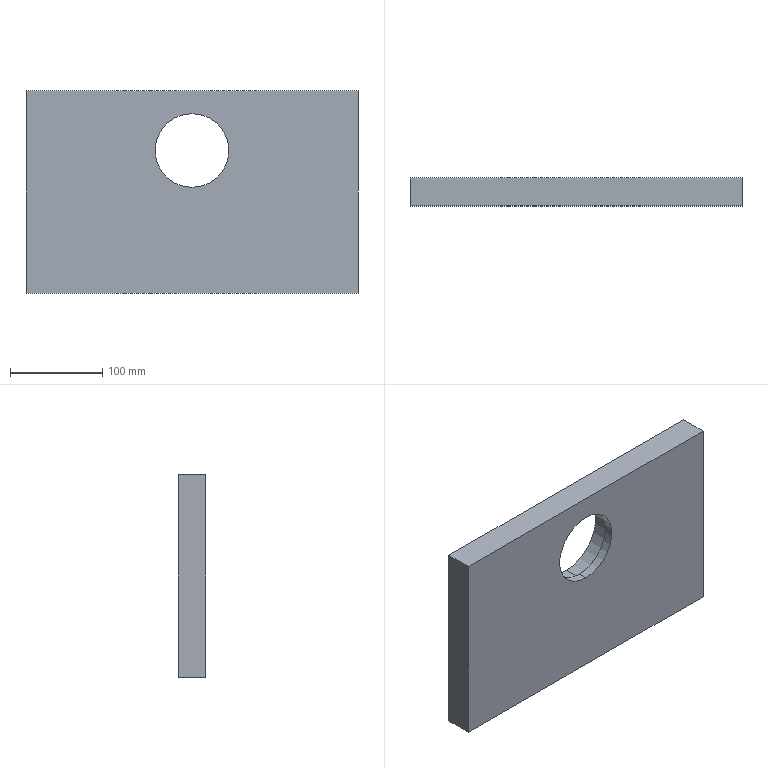Part | SolidWorks | features Cut 2, Extrusion 1 | 1 solid | 11 faces | box 360 x 30 x 220 mm | volume 2198500 mm3 | plane 7 | cylinder 4 | commonest cylinder face diameters 80 x2 90 x2
STEP:
#1=CARTESIAN_POINT('',(0.,10.,90.));
#2=VERTEX_POINT('',#1);
#3=CARTESIAN_POINT('',(0.,10.,0.));
#4=VERTEX_POINT('',#3);
#5=CARTESIAN_POINT('',(0.,10.,45.));
#6=DIRECTION('',(0.,-1.,0.));
#7=DIRECTION('',(0.,0.,-1.));
#8=AXIS2_PLACEMENT_3D('',#5,#6,#7);
#9=CIRCLE('',#8,45.);
#10=EDGE_CURVE('',#2,#4,#9,.T.);
#11=ORIENTED_EDGE('',*,*,#10,.T.);
#12=CARTESIAN_POINT('',(0.,30.,0.));
#13=VERTEX_POINT('',#12);
#14=CARTESIAN_POINT('',(0.,10.,0.));
#15=DIRECTION('',(0.,1.,0.));
#16=VECTOR('',#15,1000.);
#17=LINE('',#14,#16);
#18=EDGE_CURVE('',#4,#13,#17,.T.);
#19=ORIENTED_EDGE('',*,*,#18,.T.);
#20=CARTESIAN_POINT('',(0.,30.,90.));
#21=VERTEX_POINT('',#20);
#22=CARTESIAN_POINT('',(0.,30.,45.));
#23=DIRECTION('',(0.,-1.,0.));
#24=DIRECTION('',(0.,0.,-1.));
#25=AXIS2_PLACEMENT_3D('',#22,#23,#24);
#26=CIRCLE('',#25,45.);
#27=EDGE_CURVE('',#21,#13,#26,.T.);
#28=ORIENTED_EDGE('',*,*,#27,.F.);
#29=CARTESIAN_POINT('',(0.,10.,90.));
#30=DIRECTION('',(0.,1.,0.));
#31=VECTOR('',#30,1000.);
#32=LINE('',#29,#31);
#33=EDGE_CURVE('',#2,#21,#32,.T.);
#34=ORIENTED_EDGE('',*,*,#33,.F.);
#35=EDGE_LOOP('',(#11,#19,#28,#34));
#36=FACE_OUTER_BOUND('',#35,.T.);
#37=CARTESIAN_POINT('',(0.,10.,45.));
#38=DIRECTION('',(0.,1.,0.));
#39=DIRECTION('',(0.,0.,1.));
#40=AXIS2_PLACEMENT_3D('',#37,#38,#39);
#41=CYLINDRICAL_SURFACE('',#40,45.);
#42=ADVANCED_FACE('',(#36),#41,.F.);
#43=CARTESIAN_POINT('',(0.,0.,5.));
#44=VERTEX_POINT('',#43);
#45=CARTESIAN_POINT('',(0.,0.,85.));
#46=VERTEX_POINT('',#45);
#47=CARTESIAN_POINT('',(0.,0.,45.));
#48=DIRECTION('',(0.,1.,0.));
#49=DIRECTION('',(0.,0.,1.));
#50=AXIS2_PLACEMENT_3D('',#47,#48,#49);
#51=CIRCLE('',#50,40.);
#52=EDGE_CURVE('',#44,#46,#51,.T.);
#53=ORIENTED_EDGE('',*,*,#52,.F.);
#54=CARTESIAN_POINT('',(0.,10.,5.));
#55=VERTEX_POINT('',#54);
#56=CARTESIAN_POINT('',(0.,0.,5.));
#57=DIRECTION('',(0.,1.,0.));
#58=VECTOR('',#57,1000.);
#59=LINE('',#56,#58);
#60=EDGE_CURVE('',#44,#55,#59,.T.);
#61=ORIENTED_EDGE('',*,*,#60,.T.);
#62=CARTESIAN_POINT('',(0.,10.,85.));
#63=VERTEX_POINT('',#62);
#64=CARTESIAN_POINT('',(0.,10.,45.));
#65=DIRECTION('',(0.,1.,0.));
#66=DIRECTION('',(0.,0.,-1.));
#67=AXIS2_PLACEMENT_3D('',#64,#65,#66);
#68=CIRCLE('',#67,40.);
#69=EDGE_CURVE('',#55,#63,#68,.T.);
#70=ORIENTED_EDGE('',*,*,#69,.T.);
#71=CARTESIAN_POINT('',(0.,0.,85.));
#72=DIRECTION('',(0.,1.,0.));
#73=VECTOR('',#72,1000.);
#74=LINE('',#71,#73);
#75=EDGE_CURVE('',#46,#63,#74,.T.);
#76=ORIENTED_EDGE('',*,*,#75,.F.);
#77=EDGE_LOOP('',(#53,#61,#70,#76));
#78=FACE_OUTER_BOUND('',#77,.T.);
#79=CARTESIAN_POINT('',(0.,0.,45.));
#80=DIRECTION('',(0.,1.,0.));
#81=DIRECTION('',(0.,0.,1.));
#82=AXIS2_PLACEMENT_3D('',#79,#80,#81);
#83=CYLINDRICAL_SURFACE('',#82,40.);
#84=ADVANCED_FACE('',(#78),#83,.F.);
#85=CARTESIAN_POINT('',(180.,0.,110.));
#86=VERTEX_POINT('',#85);
#87=CARTESIAN_POINT('',(180.,0.,-110.));
#88=VERTEX_POINT('',#87);
#89=CARTESIAN_POINT('',(180.,0.,110.));
#90=DIRECTION('',(0.,0.,-1.));
#91=VECTOR('',#90,1000.);
#92=LINE('',#89,#91);
#93=EDGE_CURVE('',#86,#88,#92,.T.);
#94=ORIENTED_EDGE('',*,*,#93,.T.);
#95=CARTESIAN_POINT('',(180.,30.,-110.));
#96=VERTEX_POINT('',#95);
#97=CARTESIAN_POINT('',(180.,30.,-110.));
#98=DIRECTION('',(0.,-1.,0.));
#99=VECTOR('',#98,1000.);
#100=LINE('',#97,#99);
#101=EDGE_CURVE('',#96,#88,#100,.T.);
#102=ORIENTED_EDGE('',*,*,#101,.F.);
#103=CARTESIAN_POINT('',(180.,30.,110.));
#104=VERTEX_POINT('',#103);
#105=CARTESIAN_POINT('',(180.,30.,110.));
#106=DIRECTION('',(0.,0.,-1.));
#107=VECTOR('',#106,1000.);
#108=LINE('',#105,#107);
#109=EDGE_CURVE('',#104,#96,#108,.T.);
#110=ORIENTED_EDGE('',*,*,#109,.F.);
#111=CARTESIAN_POINT('',(180.,30.,110.));
#112=DIRECTION('',(0.,-1.,0.));
#113=VECTOR('',#112,1000.);
#114=LINE('',#111,#113);
#115=EDGE_CURVE('',#104,#86,#114,.T.);
#116=ORIENTED_EDGE('',*,*,#115,.T.);
#117=EDGE_LOOP('',(#94,#102,#110,#116));
#118=FACE_OUTER_BOUND('',#117,.T.);
#119=CARTESIAN_POINT('',(180.,30.,110.));
#120=DIRECTION('',(-1.,0.,0.));
#121=DIRECTION('',(0.,0.,1.));
#122=AXIS2_PLACEMENT_3D('',#119,#120,#121);
#123=PLANE('',#122);
#124=ADVANCED_FACE('',(#118),#123,.F.);
#125=CARTESIAN_POINT('',(-180.,0.,-110.));
#126=VERTEX_POINT('',#125);
#127=CARTESIAN_POINT('',(-180.,0.,-110.));
#128=DIRECTION('',(-1.,0.,0.));
#129=VECTOR('',#128,1000.);
#130=LINE('',#127,#129);
#131=EDGE_CURVE('',#88,#126,#130,.T.);
#132=ORIENTED_EDGE('',*,*,#131,.T.);
#133=CARTESIAN_POINT('',(-180.,30.,-110.));
#134=VERTEX_POINT('',#133);
#135=CARTESIAN_POINT('',(-180.,30.,-110.));
#136=DIRECTION('',(0.,-1.,0.));
#137=VECTOR('',#136,1000.);
#138=LINE('',#135,#137);
#139=EDGE_CURVE('',#134,#126,#138,.T.);
#140=ORIENTED_EDGE('',*,*,#139,.F.);
#141=CARTESIAN_POINT('',(-180.,30.,-110.));
#142=DIRECTION('',(-1.,0.,0.));
#143=VECTOR('',#142,1000.);
#144=LINE('',#141,#143);
#145=EDGE_CURVE('',#96,#134,#144,.T.);
#146=ORIENTED_EDGE('',*,*,#145,.F.);
#147=ORIENTED_EDGE('',*,*,#101,.T.);
#148=EDGE_LOOP('',(#132,#140,#146,#147));
#149=FACE_OUTER_BOUND('',#148,.T.);
#150=CARTESIAN_POINT('',(-180.,30.,-110.));
#151=DIRECTION('',(0.,0.,1.));
#152=DIRECTION('',(1.,0.,0.));
#153=AXIS2_PLACEMENT_3D('',#150,#151,#152);
#154=PLANE('',#153);
#155=ADVANCED_FACE('',(#149),#154,.F.);
#156=CARTESIAN_POINT('',(-180.,0.,110.));
#157=VERTEX_POINT('',#156);
#158=CARTESIAN_POINT('',(-180.,0.,110.));
#159=DIRECTION('',(0.,0.,1.));
#160=VECTOR('',#159,1000.);
#161=LINE('',#158,#160);
#162=EDGE_CURVE('',#126,#157,#161,.T.);
#163=ORIENTED_EDGE('',*,*,#162,.T.);
#164=CARTESIAN_POINT('',(-180.,30.,110.));
#165=VERTEX_POINT('',#164);
#166=CARTESIAN_POINT('',(-180.,30.,110.));
#167=DIRECTION('',(0.,-1.,0.));
#168=VECTOR('',#167,1000.);
#169=LINE('',#166,#168);
#170=EDGE_CURVE('',#165,#157,#169,.T.);
#171=ORIENTED_EDGE('',*,*,#170,.F.);
#172=CARTESIAN_POINT('',(-180.,30.,110.));
#173=DIRECTION('',(0.,0.,1.));
#174=VECTOR('',#173,1000.);
#175=LINE('',#172,#174);
#176=EDGE_CURVE('',#134,#165,#175,.T.);
#177=ORIENTED_EDGE('',*,*,#176,.F.);
#178=ORIENTED_EDGE('',*,*,#139,.T.);
#179=EDGE_LOOP('',(#163,#171,#177,#178));
#180=FACE_OUTER_BOUND('',#179,.T.);
#181=CARTESIAN_POINT('',(-180.,30.,110.));
#182=DIRECTION('',(1.,0.,0.));
#183=DIRECTION('',(0.,0.,-1.));
#184=AXIS2_PLACEMENT_3D('',#181,#182,#183);
#185=PLANE('',#184);
#186=ADVANCED_FACE('',(#180),#185,.F.);
#187=CARTESIAN_POINT('',(-180.,0.,110.));
#188=DIRECTION('',(1.,0.,0.));
#189=VECTOR('',#188,1000.);
#190=LINE('',#187,#189);
#191=EDGE_CURVE('',#157,#86,#190,.T.);
#192=ORIENTED_EDGE('',*,*,#191,.T.);
#193=ORIENTED_EDGE('',*,*,#115,.F.);
#194=CARTESIAN_POINT('',(-180.,30.,110.));
#195=DIRECTION('',(1.,0.,0.));
#196=VECTOR('',#195,1000.);
#197=LINE('',#194,#196);
#198=EDGE_CURVE('',#165,#104,#197,.T.);
#199=ORIENTED_EDGE('',*,*,#198,.F.);
#200=ORIENTED_EDGE('',*,*,#170,.T.);
#201=EDGE_LOOP('',(#192,#193,#199,#200));
#202=FACE_OUTER_BOUND('',#201,.T.);
#203=CARTESIAN_POINT('',(-180.,30.,110.));
#204=DIRECTION('',(0.,0.,-1.));
#205=DIRECTION('',(-1.,0.,0.));
#206=AXIS2_PLACEMENT_3D('',#203,#204,#205);
#207=PLANE('',#206);
#208=ADVANCED_FACE('',(#202),#207,.F.);
#209=ORIENTED_EDGE('',*,*,#27,.T.);
#210=CARTESIAN_POINT('',(0.,30.,45.));
#211=DIRECTION('',(0.,-1.,0.));
#212=DIRECTION('',(0.,0.,-1.));
#213=AXIS2_PLACEMENT_3D('',#210,#211,#212);
#214=CIRCLE('',#213,45.);
#215=EDGE_CURVE('',#13,#21,#214,.T.);
#216=ORIENTED_EDGE('',*,*,#215,.T.);
#217=EDGE_LOOP('',(#209,#216));
#218=FACE_BOUND('',#217,.T.);
#219=ORIENTED_EDGE('',*,*,#109,.T.);
#220=ORIENTED_EDGE('',*,*,#145,.T.);
#221=ORIENTED_EDGE('',*,*,#176,.T.);
#222=ORIENTED_EDGE('',*,*,#198,.T.);
#223=EDGE_LOOP('',(#219,#220,#221,#222));
#224=FACE_OUTER_BOUND('',#223,.T.);
#225=CARTESIAN_POINT('',(0.,30.,0.));
#226=DIRECTION('',(0.,-1.,0.));
#227=DIRECTION('',(0.,0.,-1.));
#228=AXIS2_PLACEMENT_3D('',#225,#226,#227);
#229=PLANE('',#228);
#230=ADVANCED_FACE('',(#218,#224),#229,.F.);
#231=CARTESIAN_POINT('',(0.,0.,45.));
#232=DIRECTION('',(0.,1.,0.));
#233=DIRECTION('',(0.,0.,1.));
#234=AXIS2_PLACEMENT_3D('',#231,#232,#233);
#235=CIRCLE('',#234,40.);
#236=EDGE_CURVE('',#46,#44,#235,.T.);
#237=ORIENTED_EDGE('',*,*,#236,.T.);
#238=ORIENTED_EDGE('',*,*,#52,.T.);
#239=EDGE_LOOP('',(#237,#238));
#240=FACE_BOUND('',#239,.T.);
#241=ORIENTED_EDGE('',*,*,#93,.F.);
#242=ORIENTED_EDGE('',*,*,#191,.F.);
#243=ORIENTED_EDGE('',*,*,#162,.F.);
#244=ORIENTED_EDGE('',*,*,#131,.F.);
#245=EDGE_LOOP('',(#241,#242,#243,#244));
#246=FACE_OUTER_BOUND('',#245,.T.);
#247=CARTESIAN_POINT('',(0.,0.,0.));
#248=DIRECTION('',(0.,-1.,0.));
#249=DIRECTION('',(0.,0.,-1.));
#250=AXIS2_PLACEMENT_3D('',#247,#248,#249);
#251=PLANE('',#250);
#252=ADVANCED_FACE('',(#240,#246),#251,.T.);
#253=ORIENTED_EDGE('',*,*,#60,.F.);
#254=ORIENTED_EDGE('',*,*,#236,.F.);
#255=ORIENTED_EDGE('',*,*,#75,.T.);
#256=CARTESIAN_POINT('',(0.,10.,45.));
#257=DIRECTION('',(0.,1.,0.));
#258=DIRECTION('',(0.,0.,-1.));
#259=AXIS2_PLACEMENT_3D('',#256,#257,#258);
#260=CIRCLE('',#259,40.);
#261=EDGE_CURVE('',#63,#55,#260,.T.);
#262=ORIENTED_EDGE('',*,*,#261,.T.);
#263=EDGE_LOOP('',(#253,#254,#255,#262));
#264=FACE_OUTER_BOUND('',#263,.T.);
#265=CARTESIAN_POINT('',(0.,0.,45.));
#266=DIRECTION('',(0.,1.,0.));
#267=DIRECTION('',(0.,0.,1.));
#268=AXIS2_PLACEMENT_3D('',#265,#266,#267);
#269=CYLINDRICAL_SURFACE('',#268,40.);
#270=ADVANCED_FACE('',(#264),#269,.F.);
#271=ORIENTED_EDGE('',*,*,#10,.F.);
#272=CARTESIAN_POINT('',(0.,10.,45.));
#273=DIRECTION('',(0.,-1.,0.));
#274=DIRECTION('',(0.,0.,-1.));
#275=AXIS2_PLACEMENT_3D('',#272,#273,#274);
#276=CIRCLE('',#275,45.);
#277=EDGE_CURVE('',#4,#2,#276,.T.);
#278=ORIENTED_EDGE('',*,*,#277,.F.);
#279=EDGE_LOOP('',(#271,#278));
#280=FACE_OUTER_BOUND('',#279,.T.);
#281=ORIENTED_EDGE('',*,*,#261,.F.);
#282=ORIENTED_EDGE('',*,*,#69,.F.);
#283=EDGE_LOOP('',(#281,#282));
#284=FACE_BOUND('',#283,.T.);
#285=CARTESIAN_POINT('',(0.,10.,45.));
#286=DIRECTION('',(0.,-1.,0.));
#287=DIRECTION('',(0.,0.,-1.));
#288=AXIS2_PLACEMENT_3D('',#285,#286,#287);
#289=PLANE('',#288);
#290=ADVANCED_FACE('',(#280,#284),#289,.F.);
#291=ORIENTED_EDGE('',*,*,#18,.F.);
#292=ORIENTED_EDGE('',*,*,#277,.T.);
#293=ORIENTED_EDGE('',*,*,#33,.T.);
#294=ORIENTED_EDGE('',*,*,#215,.F.);
#295=EDGE_LOOP('',(#291,#292,#293,#294));
#296=FACE_OUTER_BOUND('',#295,.T.);
#297=CARTESIAN_POINT('',(0.,10.,45.));
#298=DIRECTION('',(0.,1.,0.));
#299=DIRECTION('',(0.,0.,1.));
#300=AXIS2_PLACEMENT_3D('',#297,#298,#299);
#301=CYLINDRICAL_SURFACE('',#300,45.);
#302=ADVANCED_FACE('',(#296),#301,.F.);
#303=CLOSED_SHELL('',(#42,#84,#124,#155,#186,#208,#230,#252,#270,#290,#302));
#304=MANIFOLD_SOLID_BREP('',#303);
#305=CARTESIAN_POINT('',(0.,0.,0.));
#306=DIRECTION('',(0.,0.,1.));
#307=DIRECTION('',(1.,0.,0.));
#308=AXIS2_PLACEMENT_3D('',#305,#306,#307);
#309=(LENGTH_UNIT()NAMED_UNIT(*)SI_UNIT(.MILLI.,.METRE.));
#310=UNCERTAINTY_MEASURE_WITH_UNIT(LENGTH_MEASURE(0.00001),#309,'','');
#311=(NAMED_UNIT(*)PLANE_ANGLE_UNIT()SI_UNIT($,.RADIAN.));
#312=(NAMED_UNIT(*)SI_UNIT($,.STERADIAN.)SOLID_ANGLE_UNIT());
#313=(GEOMETRIC_REPRESENTATION_CONTEXT(3)GLOBAL_UNCERTAINTY_ASSIGNED_CONTEXT((#310))GLOBAL_UNIT_ASSIGNED_CONTEXT((#309,#311,#312))REPRESENTATION_CONTEXT('',''));
#314=ADVANCED_BREP_SHAPE_REPRESENTATION('',(#304,#308),#313);